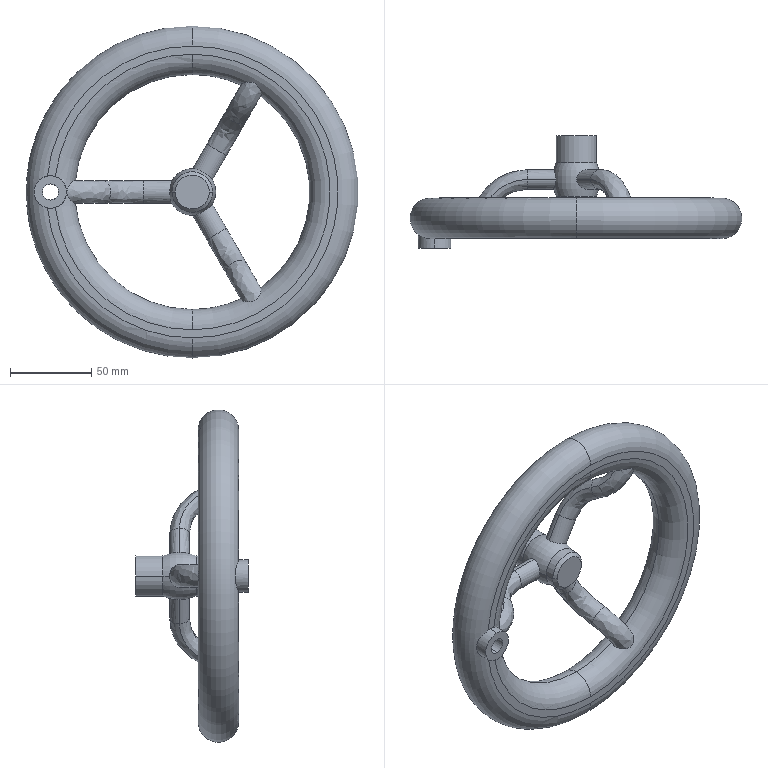Part | SolidWorks | features ICE 3, Revolution 2, CirPattern 1, Sweep 1 | 1 solid | 46 faces | box 205 x 69.5 x 205 mm | volume 388207 mm3 | spline 18 | cylinder 10 | torus 8 | plane 8 | cone 2 | commonest cylinder face diameters 25 x4 10 x2 12 x2 20 x2